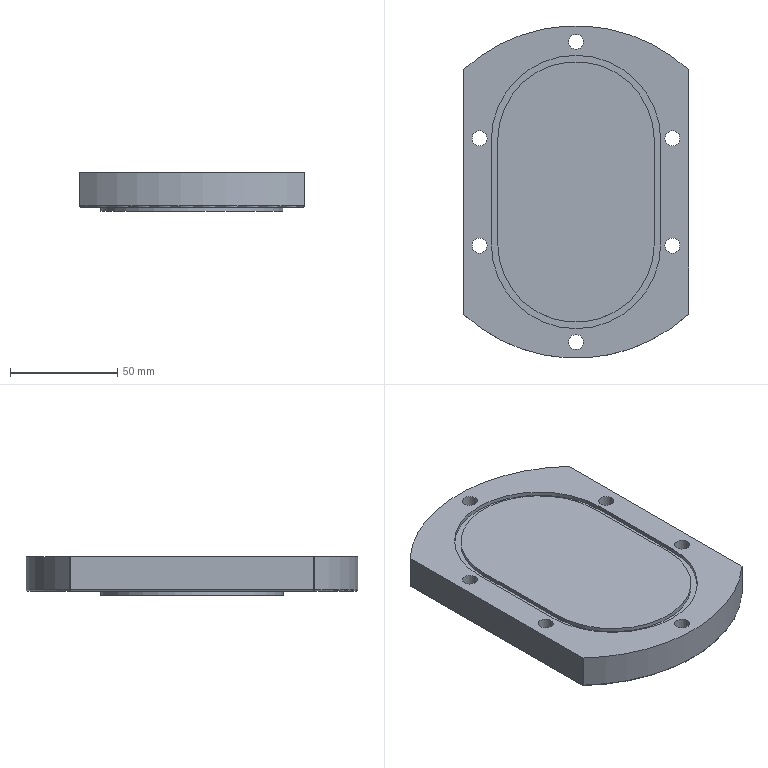NC program | NX | posted with a generic post | part box 105 x 155 x 18 mm
Whole program:
N10 G17 G21 G94 G90
(FLOOR_WALL_COPY_1_COPY , TOOL : D50)
N12 T02 M6
N14 G54
N16 G17 G0 G90 X-61.025 Y52.5 S1200 M3
N18 G43 Z30. H2
N20 Z7.65
N22 G94 G1 Z4.65 F1000.
N24 X-57.009
N26 X57.009 F2000.
N28 G2 X73.636 Y24.167 R77.5
N30 G1 X-73.636
N32 G3 X-77.388 Y-4.167 R77.5
N34 G1 X77.388
N36 G2 X70.356 Y-32.5 R77.5
N38 G1 X-70.356
N40 X-73.648
N42 Z7.65
N44 G0 Z30.
N46 X-61.025 Y52.5
N48 Z7.3
N50 G1 Z4.3 F1000.
N52 X-57.009
N54 X57.009 F2000.
N56 G2 X73.636 Y24.167 R77.5
N58 G1 X-73.636
N60 G3 X-77.388 Y-4.167 R77.5
N62 G1 X77.388
N64 G2 X70.356 Y-32.5 R77.5
N66 G1 X-70.356
N68 X-73.648
N70 Z7.3
N72 G0 Z30.
N74 X-61.025 Y52.5
N76 Z6.95
N78 G1 Z3.95 F1000.
N80 X-57.009
N82 X57.009 F2000.
N84 G2 X73.636 Y24.167 R77.5
N86 G1 X-73.636
N88 G3 X-77.388 Y-4.167 R77.5
N90 G1 X77.388
N92 G2 X70.356 Y-32.5 R77.5
N94 G1 X-70.356
N96 X-73.648
N98 Z6.95
N100 G0 Z30.
N102 X-61.025 Y52.5
N104 Z6.6
N106 G1 Z3.6 F1000.
N108 X-57.009
N110 X57.009 F2000.
N112 G2 X73.636 Y24.167 R77.5
N114 G1 X-73.636
N116 G3 X-77.388 Y-4.167 R77.5
N118 G1 X77.388
N120 G2 X70.356 Y-32.5 R77.5
N122 G1 X-70.356
N124 X-73.648
N126 Z6.6
N128 G0 Z30.
N130 X-61.025 Y52.5
N132 Z6.25
N134 G1 Z3.25 F1000.
N136 X-57.009
N138 X57.009 F2000.
N140 G2 X73.636 Y24.167 R77.5
N142 G1 X-73.636
N144 G3 X-77.388 Y-4.167 R77.5
N146 G1 X77.388
N148 G2 X70.356 Y-32.5 R77.5
N150 G1 X-70.356
N152 X-73.648
N154 Z6.25
N156 G0 Z30.
N158 X-61.025 Y52.5
N160 Z5.9
N162 G1 Z2.9 F1000.
N164 X-57.009
N166 X57.009 F2000.
N168 G2 X73.636 Y24.167 R77.5
N170 G1 X-73.636
N172 G3 X-77.388 Y-4.167 R77.5
N174 G1 X77.388
N176 G2 X70.356 Y-32.5 R77.5
N178 G1 X-70.356
N180 X-73.648
N182 Z5.9
N184 G0 Z30.
N186 X-61.025 Y52.5
N188 Z5.55
N190 G1 Z2.55 F1000.
N192 X-57.009
N194 X57.009 F2000.
N196 G2 X73.636 Y24.167 R77.5
N198 G1 X-73.636
N200 G3 X-77.388 Y-4.167 R77.5
N202 G1 X77.388
N204 G2 X70.356 Y-32.5 R77.5
N206 G1 X-70.356
N208 X-73.648
N210 Z5.55
N212 G0 Z30.
N214 X-61.025 Y52.5
N216 Z5.2
N218 G1 Z2.2 F1000.
N220 X-57.009
N222 X57.009 F2000.
N224 G2 X73.636 Y24.167 R77.5
N226 G1 X-73.636
N228 G3 X-77.388 Y-4.167 R77.5
N230 G1 X77.388
N232 G2 X70.356 Y-32.5 R77.5
N234 G1 X-70.356
N236 X-73.648
N238 Z5.2
N240 G0 Z30.
N242 X-61.025 Y52.5
N244 Z4.85
N246 G1 Z1.85 F1000.
N248 X-57.009
N250 X57.009 F2000.
N252 G2 X73.636 Y24.167 R77.5
N254 G1 X-73.636
N256 G3 X-77.388 Y-4.167 R77.5
N258 G1 X77.388
N260 G2 X70.356 Y-32.5 R77.5
N262 G1 X-70.356
N264 X-73.648
N266 Z4.85
N268 G0 Z30.
N270 X-61.025 Y52.5
N272 Z4.5
N274 G1 Z1.5 F1000.
N276 X-57.009
N278 X57.009 F2000.
N280 G2 X73.636 Y24.167 R77.5
N282 G1 X-73.636
N284 G3 X-77.388 Y-4.167 R77.5
N286 G1 X77.388
N288 G2 X70.356 Y-32.5 R77.5
N290 G1 X-70.356
N292 X-73.648
N294 Z4.5
N296 G0 Z30.
N298 X-61.025 Y52.5
N300 Z4.15
N302 G1 Z1.15 F1000.
N304 X-57.009
N306 X57.009 F2000.
N308 G2 X73.636 Y24.167 R77.5
N310 G1 X-73.636
N312 G3 X-77.388 Y-4.167 R77.5
N314 G1 X77.388
N316 G2 X70.356 Y-32.5 R77.5
N318 G1 X-70.356
N320 X-73.648
N322 Z4.15
N324 G0 Z30.
N326 X-61.025 Y52.5
N328 Z3.8
N330 G1 Z0.8 F1000.
N332 X-57.009
N334 X57.009 F2000.
N336 G2 X73.636 Y24.167 R77.5
N338 G1 X-73.636
N340 G3 X-77.388 Y-4.167 R77.5
N342 G1 X77.388
N344 G2 X70.356 Y-32.5 R77.5
N346 G1 X-70.356
N348 X-73.648
N350 Z3.8
N352 G0 Z30.
N354 X-61.025 Y52.5
N356 Z3.45
N358 G1 Z0.45 F1000.
N360 X-57.009
N362 X57.009 F2000.
N364 G2 X73.636 Y24.167 R77.5
N366 G1 X-73.636
N368 G3 X-77.388 Y-4.167 R77.5
N370 G1 X77.388
N372 G2 X70.356 Y-32.5 R77.5
N374 G1 X-70.356
N376 X-73.648
N378 Z3.45
N380 G0 Z30.
N382 X-61.025 Y52.5
N384 Z3.1
N386 G1 Z0.1 F1000.
N388 X-57.009
N390 X57.009 F2000.
N392 G2 X73.636 Y24.167 R77.5
N394 G1 X-73.636
N396 G3 X-77.388 Y-4.167 R77.5
N398 G1 X77.388
N400 G2 X70.356 Y-32.5 R77.5
N402 G1 X-70.356
N404 X-73.648
N406 Z3.1
N408 G0 Z30.
(FLOOR_WALL_COPY_COPY_COPY , TOOL : D50)
N410 X-61.025 Y52.5 S2500
N412 Z3.
N414 G1 Z0. F1000.
N416 X-57.009
N418 X57.009
N420 G2 X73.636 Y24.167 R77.5
N422 G1 X-73.636
N424 G3 X-77.388 Y-4.167 R77.5
N426 G1 X77.388
N428 G2 X70.356 Y-32.5 R77.5
N430 G1 X-70.356
N432 X-73.648
N434 Z3.
N436 G0 Z30.
N438 M5
(HOLE_MILLING_COPY_COPY , TOOL : D6)
N440 T06 M6
N442 G54
N444 G17 G0 G90 X-25. Y45. S4987 M3
N446 G43 Z30. H6
N448 Z-1.
N450 G94 G3 X-23.75 Y46.25 R1.25 F1500.
N452 X-25. Y47.5 R1.25
N454 X-25. Y47.5 Z-1.1 I0. J-2.5
N456 X-25. Y47.5 Z-1.2 I0. J-2.5
N458 X-25. Y47.5 Z-1.3 I0. J-2.5
N460 X-25. Y47.5 Z-1.4 I0. J-2.5
N462 X-25. Y47.5 Z-1.5 I0. J-2.5
N464 X-25. Y47.5 Z-1.6 I0. J-2.5
N466 X-25. Y47.5 Z-1.7 I0. J-2.5
N468 X-25. Y47.5 Z-1.8 I0. J-2.5
N470 X-25. Y47.5 Z-1.9 I0. J-2.5
N472 X-25. Y47.5 Z-2. I0. J-2.5
N474 X-25. Y47.5 Z-2.1 I0. J-2.5
N476 X-25. Y47.5 Z-2.2 I0. J-2.5
N478 X-25. Y47.5 Z-2.3 I0. J-2.5
N480 X-25. Y47.5 Z-2.4 I0. J-2.5
N482 X-25. Y47.5 Z-2.5 I0. J-2.5
N484 X-25. Y47.5 Z-2.6 I0. J-2.5
N486 X-25. Y47.5 Z-2.7 I0. J-2.5
N488 X-25. Y47.5 Z-2.8 I0. J-2.5
N490 X-25. Y47.5 Z-2.9 I0. J-2.5
N492 X-25. Y47.5 Z-3. I0. J-2.5
N494 X-25. Y47.5 Z-3.1 I0. J-2.5
N496 X-25. Y47.5 Z-3.2 I0. J-2.5
N498 X-25. Y47.5 Z-3.3 I0. J-2.5
N500 X-25. Y47.5 Z-3.4 I0. J-2.5
N502 X-25. Y47.5 Z-3.5 I0. J-2.5
N504 X-25. Y47.5 Z-3.6 I0. J-2.5
N506 X-25. Y47.5 Z-3.7 I0. J-2.5
N508 X-25. Y47.5 Z-3.8 I0. J-2.5
N510 X-25. Y47.5 Z-3.9 I0. J-2.5
N512 X-25. Y47.5 Z-4. I0. J-2.5
N514 X-25. Y47.5 Z-4.1 I0. J-2.5
N516 X-25. Y47.5 Z-4.2 I0. J-2.5
N518 X-25. Y47.5 Z-4.3 I0. J-2.5
N520 X-25. Y47.5 Z-4.4 I0. J-2.5
N522 X-25. Y47.5 Z-4.5 I0. J-2.5
N524 X-25. Y47.5 Z-4.6 I0. J-2.5
N526 X-25. Y47.5 Z-4.7 I0. J-2.5
N528 X-25. Y47.5 Z-4.8 I0. J-2.5
N530 X-25. Y47.5 Z-4.9 I0. J-2.5
N532 X-25. Y47.5 Z-5. I0. J-2.5
N534 X-25. Y47.5 Z-5.1 I0. J-2.5
N536 X-25. Y47.5 Z-5.2 I0. J-2.5
N538 X-25. Y47.5 Z-5.3 I0. J-2.5
N540 X-25. Y47.5 Z-5.4 I0. J-2.5
N542 X-25. Y47.5 Z-5.5 I0. J-2.5
N544 X-25. Y47.5 Z-5.6 I0. J-2.5
N546 X-25. Y47.5 Z-5.7 I0. J-2.5
N548 X-25. Y47.5 Z-5.8 I0. J-2.5
N550 X-25. Y47.5 Z-5.9 I0. J-2.5
N552 X-25. Y47.5 Z-6. I0. J-2.5
N554 X-25. Y47.5 Z-6.1 I0. J-2.5
N556 X-25. Y47.5 Z-6.2 I0. J-2.5
N558 X-25. Y47.5 Z-6.3 I0. J-2.5
N560 X-25. Y47.5 Z-6.4 I0. J-2.5
N562 X-25. Y47.5 Z-6.5 I0. J-2.5
N564 X-25. Y47.5 Z-6.6 I0. J-2.5
N566 X-25. Y47.5 Z-6.7 I0. J-2.5
N568 X-25. Y47.5 Z-6.8 I0. J-2.5
N570 X-25. Y47.5 Z-6.9 I0. J-2.5
N572 X-25. Y47.5 Z-7. I0. J-2.5
N574 X-25. Y47.5 Z-7.1 I0. J-2.5
N576 X-25. Y47.5 Z-7.2 I0. J-2.5
N578 X-25. Y47.5 Z-7.3 I0. J-2.5
N580 X-25. Y47.5 Z-7.4 I0. J-2.5
N582 X-25. Y47.5 Z-7.5 I0. J-2.5
N584 X-25. Y47.5 Z-7.6 I0. J-2.5
N586 X-25. Y47.5 Z-7.7 I0. J-2.5
N588 X-25. Y47.5 Z-7.8 I0. J-2.5
N590 X-25. Y47.5 Z-7.9 I0. J-2.5
N592 X-25. Y47.5 Z-8. I0. J-2.5
N594 X-25. Y47.5 Z-8.1 I0. J-2.5
N596 X-25. Y47.5 Z-8.2 I0. J-2.5
N598 X-25. Y47.5 Z-8.3 I0. J-2.5
N600 X-25. Y47.5 Z-8.4 I0. J-2.5
N602 X-25. Y47.5 Z-8.5 I0. J-2.5
N604 X-25. Y47.5 Z-8.6 I0. J-2.5
N606 X-25. Y47.5 Z-8.7 I0. J-2.5
N608 X-25. Y47.5 Z-8.8 I0. J-2.5
N610 X-27.5 Y45. R2.5
N612 X-25. Y47.5 R-2.5
N614 X-26.25 Y46.25 R1.25
N616 X-25. Y45. R1.25
N618 G0 Z30.
N620 X-70. Y0.
N622 Z-1.
N624 G3 X-68.75 Y1.25 R1.25
N626 X-70. Y2.5 R1.25
N628 X-70. Y2.5 Z-1.1 I0. J-2.5
N630 X-70. Y2.5 Z-1.2 I0. J-2.5
N632 X-70. Y2.5 Z-1.3 I0. J-2.5
N634 X-70. Y2.5 Z-1.4 I0. J-2.5
N636 X-70. Y2.5 Z-1.5 I0. J-2.5
N638 X-70. Y2.5 Z-1.6 I0. J-2.5
N640 X-70. Y2.5 Z-1.7 I0. J-2.5
N642 X-70. Y2.5 Z-1.8 I0. J-2.5
N644 X-70. Y2.5 Z-1.9 I0. J-2.5
N646 X-70. Y2.5 Z-2. I0. J-2.5
N648 X-70. Y2.5 Z-2.1 I0. J-2.5
N650 X-70. Y2.5 Z-2.2 I0. J-2.5
N652 X-70. Y2.5 Z-2.3 I0. J-2.5
N654 X-70. Y2.5 Z-2.4 I0. J-2.5
N656 X-70. Y2.5 Z-2.5 I0. J-2.5
N658 X-70. Y2.5 Z-2.6 I0. J-2.5
N660 X-70. Y2.5 Z-2.7 I0. J-2.5
N662 X-70. Y2.5 Z-2.8 I0. J-2.5
N664 X-70. Y2.5 Z-2.9 I0. J-2.5
N666 X-70. Y2.5 Z-3. I0. J-2.5
N668 X-70. Y2.5 Z-3.1 I0. J-2.5
N670 X-70. Y2.5 Z-3.2 I0. J-2.5
N672 X-70. Y2.5 Z-3.3 I0. J-2.5
N674 X-70. Y2.5 Z-3.4 I0. J-2.5
N676 X-70. Y2.5 Z-3.5 I0. J-2.5
N678 X-70. Y2.5 Z-3.6 I0. J-2.5
N680 X-70. Y2.5 Z-3.7 I0. J-2.5
N682 X-70. Y2.5 Z-3.8 I0. J-2.5
N684 X-70. Y2.5 Z-3.9 I0. J-2.5
N686 X-70. Y2.5 Z-4. I0. J-2.5
N688 X-70. Y2.5 Z-4.1 I0. J-2.5
N690 X-70. Y2.5 Z-4.2 I0. J-2.5
N692 X-70. Y2.5 Z-4.3 I0. J-2.5
N694 X-70. Y2.5 Z-4.4 I0. J-2.5
N696 X-70. Y2.5 Z-4.5 I0. J-2.5
N698 X-70. Y2.5 Z-4.6 I0. J-2.5
N700 X-70. Y2.5 Z-4.7 I0. J-2.5
N702 X-70. Y2.5 Z-4.8 I0. J-2.5
N704 X-70. Y2.5 Z-4.9 I0. J-2.5
N706 X-70. Y2.5 Z-5. I0. J-2.5
N708 X-70. Y2.5 Z-5.1 I0. J-2.5
N710 X-70. Y2.5 Z-5.2 I0. J-2.5
N712 X-70. Y2.5 Z-5.3 I0. J-2.5
N714 X-70. Y2.5 Z-5.4 I0. J-2.5
N716 X-70. Y2.5 Z-5.5 I0. J-2.5
N718 X-70. Y2.5 Z-5.6 I0. J-2.5
N720 X-70. Y2.5 Z-5.7 I0. J-2.5
N722 X-70. Y2.5 Z-5.8 I0. J-2.5
N724 X-70. Y2.5 Z-5.9 I0. J-2.5
N726 X-70. Y2.5 Z-6. I0. J-2.5
N728 X-70. Y2.5 Z-6.1 I0. J-2.5
N730 X-70. Y2.5 Z-6.2 I0. J-2.5
N732 X-70. Y2.5 Z-6.3 I0. J-2.5
N734 X-70. Y2.5 Z-6.4 I0. J-2.5
N736 X-70. Y2.5 Z-6.5 I0. J-2.5
N738 X-70. Y2.5 Z-6.6 I0. J-2.5
N740 X-70. Y2.5 Z-6.7 I0. J-2.5
N742 X-70. Y2.5 Z-6.8 I0. J-2.5
N744 X-70. Y2.5 Z-6.9 I0. J-2.5
N746 X-70. Y2.5 Z-7. I0. J-2.5
N748 X-70. Y2.5 Z-7.1 I0. J-2.5
N750 X-70. Y2.5 Z-7.2 I0. J-2.5
N752 X-70. Y2.5 Z-7.3 I0. J-2.5
N754 X-70. Y2.5 Z-7.4 I0. J-2.5
N756 X-70. Y2.5 Z-7.5 I0. J-2.5
N758 X-70. Y2.5 Z-7.6 I0. J-2.5
N760 X-70. Y2.5 Z-7.7 I0. J-2.5
N762 X-70. Y2.5 Z-7.8 I0. J-2.5
N764 X-70. Y2.5 Z-7.9 I0. J-2.5
N766 X-70. Y2.5 Z-8. I0. J-2.5
N768 X-70. Y2.5 Z-8.1 I0. J-2.5
N770 X-70. Y2.5 Z-8.2 I0. J-2.5
N772 X-70. Y2.5 Z-8.3 I0. J-2.5
N774 X-70. Y2.5 Z-8.4 I0. J-2.5
N776 X-70. Y2.5 Z-8.5 I0. J-2.5
N778 X-70. Y2.5 Z-8.6 I0. J-2.5
N780 X-70. Y2.5 Z-8.7 I0. J-2.5
N782 X-70. Y2.5 Z-8.8 I0. J-2.5
N784 X-72.5 Y0. R2.5
N786 X-70. Y2.5 R-2.5
N788 X-71.25 Y1.25 R1.25
N790 X-70. Y0. R1.25
N792 G0 Z30.
N794 X25. Y45.
N796 Z-1.
N798 G3 X26.25 Y46.25 R1.25
N800 X25. Y47.5 R1.25
N802 X25. Y47.5 Z-1.1 I0. J-2.5
N804 X25. Y47.5 Z-1.2 I0. J-2.5
N806 X25. Y47.5 Z-1.3 I0. J-2.5
N808 X25. Y47.5 Z-1.4 I0. J-2.5
N810 X25. Y47.5 Z-1.5 I0. J-2.5
N812 X25. Y47.5 Z-1.6 I0. J-2.5
N814 X25. Y47.5 Z-1.7 I0. J-2.5
N816 X25. Y47.5 Z-1.8 I0. J-2.5
N818 X25. Y47.5 Z-1.9 I0. J-2.5
N820 X25. Y47.5 Z-2. I0. J-2.5
N822 X25. Y47.5 Z-2.1 I0. J-2.5
N824 X25. Y47.5 Z-2.2 I0. J-2.5
N826 X25. Y47.5 Z-2.3 I0. J-2.5
N828 X25. Y47.5 Z-2.4 I0. J-2.5
N830 X25. Y47.5 Z-2.5 I0. J-2.5
N832 X25. Y47.5 Z-2.6 I0. J-2.5
N834 X25. Y47.5 Z-2.7 I0. J-2.5
N836 X25. Y47.5 Z-2.8 I0. J-2.5
N838 X25. Y47.5 Z-2.9 I0. J-2.5
N840 X25. Y47.5 Z-3. I0. J-2.5
N842 X25. Y47.5 Z-3.1 I0. J-2.5
N844 X25. Y47.5 Z-3.2 I0. J-2.5
N846 X25. Y47.5 Z-3.3 I0. J-2.5
N848 X25. Y47.5 Z-3.4 I0. J-2.5
N850 X25. Y47.5 Z-3.5 I0. J-2.5
N852 X25. Y47.5 Z-3.6 I0. J-2.5
N854 X25. Y47.5 Z-3.7 I0. J-2.5
N856 X25. Y47.5 Z-3.8 I0. J-2.5
N858 X25. Y47.5 Z-3.9 I0. J-2.5
N860 X25. Y47.5 Z-4. I0. J-2.5
N862 X25. Y47.5 Z-4.1 I0. J-2.5
N864 X25. Y47.5 Z-4.2 I0. J-2.5
N866 X25. Y47.5 Z-4.3 I0. J-2.5
N868 X25. Y47.5 Z-4.4 I0. J-2.5
N870 X25. Y47.5 Z-4.5 I0. J-2.5
N872 X25. Y47.5 Z-4.6 I0. J-2.5
N874 X25. Y47.5 Z-4.7 I0. J-2.5
N876 X25. Y47.5 Z-4.8 I0. J-2.5
N878 X25. Y47.5 Z-4.9 I0. J-2.5
N880 X25. Y47.5 Z-5. I0. J-2.5
N882 X25. Y47.5 Z-5.1 I0. J-2.5
N884 X25. Y47.5 Z-5.2 I0. J-2.5
N886 X25. Y47.5 Z-5.3 I0. J-2.5
N888 X25. Y47.5 Z-5.4 I0. J-2.5
N890 X25. Y47.5 Z-5.5 I0. J-2.5
N892 X25. Y47.5 Z-5.6 I0. J-2.5
N894 X25. Y47.5 Z-5.7 I0. J-2.5
N896 X25. Y47.5 Z-5.8 I0. J-2.5
N898 X25. Y47.5 Z-5.9 I0. J-2.5
N900 X25. Y47.5 Z-6. I0. J-2.5
N902 X25. Y47.5 Z-6.1 I0. J-2.5
N904 X25. Y47.5 Z-6.2 I0. J-2.5
N906 X25. Y47.5 Z-6.3 I0. J-2.5
N908 X25. Y47.5 Z-6.4 I0. J-2.5
N910 X25. Y47.5 Z-6.5 I0. J-2.5
N912 X25. Y47.5 Z-6.6 I0. J-2.5
N914 X25. Y47.5 Z-6.7 I0. J-2.5
N916 X25. Y47.5 Z-6.8 I0. J-2.5
N918 X25. Y47.5 Z-6.9 I0. J-2.5
N920 X25. Y47.5 Z-7. I0. J-2.5
N922 X25. Y47.5 Z-7.1 I0. J-2.5
N924 X25. Y47.5 Z-7.2 I0. J-2.5
N926 X25. Y47.5 Z-7.3 I0. J-2.5
N928 X25. Y47.5 Z-7.4 I0. J-2.5
N930 X25. Y47.5 Z-7.5 I0. J-2.5
N932 X25. Y47.5 Z-7.6 I0. J-2.5
N934 X25. Y47.5 Z-7.7 I0. J-2.5
N936 X25. Y47.5 Z-7.8 I0. J-2.5
N938 X25. Y47.5 Z-7.9 I0. J-2.5
N940 X25. Y47.5 Z-8. I0. J-2.5
N942 X25. Y47.5 Z-8.1 I0. J-2.5
N944 X25. Y47.5 Z-8.2 I0. J-2.5
N946 X25. Y47.5 Z-8.3 I0. J-2.5
N948 X25. Y47.5 Z-8.4 I0. J-2.5
N950 X25. Y47.5 Z-8.5 I0. J-2.5
N952 X25. Y47.5 Z-8.6 I0. J-2.5
N954 X25. Y47.5 Z-8.7 I0. J-2.5
N956 X25. Y47.5 Z-8.8 I0. J-2.5
N958 X22.5 Y45. R2.5
N960 X25. Y47.5 R-2.5
N962 X23.75 Y46.25 R1.25
N964 X25. Y45. R1.25
N966 G0 Z30.
N968 X70. Y0.
N970 Z-1.
N972 G3 X71.25 Y1.25 R1.25
N974 X70. Y2.5 R1.25
N976 X70. Y2.5 Z-1.1 I0. J-2.5
N978 X70. Y2.5 Z-1.2 I0. J-2.5
N980 X70. Y2.5 Z-1.3 I0. J-2.5
N982 X70. Y2.5 Z-1.4 I0. J-2.5
N984 X70. Y2.5 Z-1.5 I0. J-2.5
N986 X70. Y2.5 Z-1.6 I0. J-2.5
N988 X70. Y2.5 Z-1.7 I0. J-2.5
N990 X70. Y2.5 Z-1.8 I0. J-2.5
N992 X70. Y2.5 Z-1.9 I0. J-2.5
N994 X70. Y2.5 Z-2. I0. J-2.5
N996 X70. Y2.5 Z-2.1 I0. J-2.5
N998 X70. Y2.5 Z-2.2 I0. J-2.5
N1000 X70. Y2.5 Z-2.3 I0. J-2.5
N1002 X70. Y2.5 Z-2.4 I0. J-2.5
N1004 X70. Y2.5 Z-2.5 I0. J-2.5
N1006 X70. Y2.5 Z-2.6 I0. J-2.5
N1008 X70. Y2.5 Z-2.7 I0. J-2.5
N1010 X70. Y2.5 Z-2.8 I0. J-2.5
N1012 X70. Y2.5 Z-2.9 I0. J-2.5
N1014 X70. Y2.5 Z-3. I0. J-2.5
N1016 X70. Y2.5 Z-3.1 I0. J-2.5
N1018 X70. Y2.5 Z-3.2 I0. J-2.5
N1020 X70. Y2.5 Z-3.3 I0. J-2.5
N1022 X70. Y2.5 Z-3.4 I0. J-2.5
N1024 X70. Y2.5 Z-3.5 I0. J-2.5
N1026 X70. Y2.5 Z-3.6 I0. J-2.5
N1028 X70. Y2.5 Z-3.7 I0. J-2.5
N1030 X70. Y2.5 Z-3.8 I0. J-2.5
N1032 X70. Y2.5 Z-3.9 I0. J-2.5
N1034 X70. Y2.5 Z-4. I0. J-2.5
N1036 X70. Y2.5 Z-4.1 I0. J-2.5
N1038 X70. Y2.5 Z-4.2 I0. J-2.5
N1040 X70. Y2.5 Z-4.3 I0. J-2.5
N1042 X70. Y2.5 Z-4.4 I0. J-2.5
N1044 X70. Y2.5 Z-4.5 I0. J-2.5
N1046 X70. Y2.5 Z-4.6 I0. J-2.5
N1048 X70. Y2.5 Z-4.7 I0. J-2.5
N1050 X70. Y2.5 Z-4.8 I0. J-2.5
N1052 X70. Y2.5 Z-4.9 I0. J-2.5
N1054 X70. Y2.5 Z-5. I0. J-2.5
N1056 X70. Y2.5 Z-5.1 I0. J-2.5
N1058 X70. Y2.5 Z-5.2 I0. J-2.5
N1060 X70. Y2.5 Z-5.3 I0. J-2.5
N1062 X70. Y2.5 Z-5.4 I0. J-2.5
N1064 X70. Y2.5 Z-5.5 I0. J-2.5
N1066 X70. Y2.5 Z-5.6 I0. J-2.5
N1068 X70. Y2.5 Z-5.7 I0. J-2.5
N1070 X70. Y2.5 Z-5.8 I0. J-2.5
N1072 X70. Y2.5 Z-5.9 I0. J-2.5
N1074 X70. Y2.5 Z-6. I0. J-2.5
N1076 X70. Y2.5 Z-6.1 I0. J-2.5
N1078 X70. Y2.5 Z-6.2 I0. J-2.5
N1080 X70. Y2.5 Z-6.3 I0. J-2.5
N1082 X70. Y2.5 Z-6.4 I0. J-2.5
N1084 X70. Y2.5 Z-6.5 I0. J-2.5
N1086 X70. Y2.5 Z-6.6 I0. J-2.5
N1088 X70. Y2.5 Z-6.7 I0. J-2.5
N1090 X70. Y2.5 Z-6.8 I0. J-2.5
N1092 X70. Y2.5 Z-6.9 I0. J-2.5
N1094 X70. Y2.5 Z-7. I0. J-2.5
N1096 X70. Y2.5 Z-7.1 I0. J-2.5
N1098 X70. Y2.5 Z-7.2 I0. J-2.5
N1100 X70. Y2.5 Z-7.3 I0. J-2.5
N1102 X70. Y2.5 Z-7.4 I0. J-2.5
N1104 X70. Y2.5 Z-7.5 I0. J-2.5
N1106 X70. Y2.5 Z-7.6 I0. J-2.5
N1108 X70. Y2.5 Z-7.7 I0. J-2.5
N1110 X70. Y2.5 Z-7.8 I0. J-2.5
N1112 X70. Y2.5 Z-7.9 I0. J-2.5
N1114 X70. Y2.5 Z-8. I0. J-2.5
N1116 X70. Y2.5 Z-8.1 I0. J-2.5
N1118 X70. Y2.5 Z-8.2 I0. J-2.5
N1120 X70. Y2.5 Z-8.3 I0. J-2.5
N1122 X70. Y2.5 Z-8.4 I0. J-2.5
N1124 X70. Y2.5 Z-8.5 I0. J-2.5
N1126 X70. Y2.5 Z-8.6 I0. J-2.5
N1128 X70. Y2.5 Z-8.7 I0. J-2.5
N1130 X70. Y2.5 Z-8.8 I0. J-2.5
N1132 X67.5 Y0. R2.5
N1134 X70. Y2.5 R-2.5
N1136 X68.75 Y1.25 R1.25
N1138 X70. Y0. R1.25
N1140 G0 Z30.
N1142 X25. Y-45.
N1144 Z-1.
N1146 G3 X26.25 Y-43.75 R1.25
N1148 X25. Y-42.5 R1.25
N1150 X25. Y-42.5 Z-1.1 I0. J-2.5
N1152 X25. Y-42.5 Z-1.2 I0. J-2.5
N1154 X25. Y-42.5 Z-1.3 I0. J-2.5
N1156 X25. Y-42.5 Z-1.4 I0. J-2.5
N1158 X25. Y-42.5 Z-1.5 I0. J-2.5
N1160 X25. Y-42.5 Z-1.6 I0. J-2.5
N1162 X25. Y-42.5 Z-1.7 I0. J-2.5
N1164 X25. Y-42.5 Z-1.8 I0. J-2.5
N1166 X25. Y-42.5 Z-1.9 I0. J-2.5
N1168 X25. Y-42.5 Z-2. I0. J-2.5
N1170 X25. Y-42.5 Z-2.1 I0. J-2.5
N1172 X25. Y-42.5 Z-2.2 I0. J-2.5
N1174 X25. Y-42.5 Z-2.3 I0. J-2.5
N1176 X25. Y-42.5 Z-2.4 I0. J-2.5
N1178 X25. Y-42.5 Z-2.5 I0. J-2.5
N1180 X25. Y-42.5 Z-2.6 I0. J-2.5
N1182 X25. Y-42.5 Z-2.7 I0. J-2.5
N1184 X25. Y-42.5 Z-2.8 I0. J-2.5
N1186 X25. Y-42.5 Z-2.9 I0. J-2.5
N1188 X25. Y-42.5 Z-3. I0. J-2.5
N1190 X25. Y-42.5 Z-3.1 I0. J-2.5
N1192 X25. Y-42.5 Z-3.2 I0. J-2.5
N1194 X25. Y-42.5 Z-3.3 I0. J-2.5
N1196 X25. Y-42.5 Z-3.4 I0. J-2.5
N1198 X25. Y-42.5 Z-3.5 I0. J-2.5
N1200 X25. Y-42.5 Z-3.6 I0. J-2.5
N1202 X25. Y-42.5 Z-3.7 I0. J-2.5
N1204 X25. Y-42.5 Z-3.8 I0. J-2.5
N1206 X25. Y-42.5 Z-3.9 I0. J-2.5
N1208 X25. Y-42.5 Z-4. I0. J-2.5
N1210 X25. Y-42.5 Z-4.1 I0. J-2.5
N1212 X25. Y-42.5 Z-4.2 I0. J-2.5
N1214 X25. Y-42.5 Z-4.3 I0. J-2.5
N1216 X25. Y-42.5 Z-4.4 I0. J-2.5
N1218 X25. Y-42.5 Z-4.5 I0. J-2.5
N1220 X25. Y-42.5 Z-4.6 I0. J-2.5
N1222 X25. Y-42.5 Z-4.7 I0. J-2.5
N1224 X25. Y-42.5 Z-4.8 I0. J-2.5
N1226 X25. Y-42.5 Z-4.9 I0. J-2.5
N1228 X25. Y-42.5 Z-5. I0. J-2.5
N1230 X25. Y-42.5 Z-5.1 I0. J-2.5
N1232 X25. Y-42.5 Z-5.2 I0. J-2.5
N1234 X25. Y-42.5 Z-5.3 I0. J-2.5
N1236 X25. Y-42.5 Z-5.4 I0. J-2.5
N1238 X25. Y-42.5 Z-5.5 I0. J-2.5
N1240 X25. Y-42.5 Z-5.6 I0. J-2.5
N1242 X25. Y-42.5 Z-5.7 I0. J-2.5
N1244 X25. Y-42.5 Z-5.8 I0. J-2.5
N1246 X25. Y-42.5 Z-5.9 I0. J-2.5
N1248 X25. Y-42.5 Z-6. I0. J-2.5
N1250 X25. Y-42.5 Z-6.1 I0. J-2.5
N1252 X25. Y-42.5 Z-6.2 I0. J-2.5
N1254 X25. Y-42.5 Z-6.3 I0. J-2.5
N1256 X25. Y-42.5 Z-6.4 I0. J-2.5
N1258 X25. Y-42.5 Z-6.5 I0. J-2.5
N1260 X25. Y-42.5 Z-6.6 I0. J-2.5
N1262 X25. Y-42.5 Z-6.7 I0. J-2.5
N1264 X25. Y-42.5 Z-6.8 I0. J-2.5
N1266 X25. Y-42.5 Z-6.9 I0. J-2.5
N1268 X25. Y-42.5 Z-7. I0. J-2.5
N1270 X25. Y-42.5 Z-7.1 I0. J-2.5
N1272 X25. Y-42.5 Z-7.2 I0. J-2.5
N1274 X25. Y-42.5 Z-7.3 I0. J-2.5
N1276 X25. Y-42.5 Z-7.4 I0. J-2.5
N1278 X25. Y-42.5 Z-7.5 I0. J-2.5
N1280 X25. Y-42.5 Z-7.6 I0. J-2.5
N1282 X25. Y-42.5 Z-7.7 I0. J-2.5
N1284 X25. Y-42.5 Z-7.8 I0. J-2.5
N1286 X25. Y-42.5 Z-7.9 I0. J-2.5
N1288 X25. Y-42.5 Z-8. I0. J-2.5
N1290 X25. Y-42.5 Z-8.1 I0. J-2.5
N1292 X25. Y-42.5 Z-8.2 I0. J-2.5
N1294 X25. Y-42.5 Z-8.3 I0. J-2.5
N1296 X25. Y-42.5 Z-8.4 I0. J-2.5
N1298 X25. Y-42.5 Z-8.5 I0. J-2.5
N1300 X25. Y-42.5 Z-8.6 I0. J-2.5
N1302 X25. Y-42.5 Z-8.7 I0. J-2.5
N1304 X25. Y-42.5 Z-8.8 I0. J-2.5
N1306 X22.5 Y-45. R2.5
N1308 X25. Y-42.5 R-2.5
N1310 X23.75 Y-43.75 R1.25
N1312 X25. Y-45. R1.25
N1314 G0 Z30.
N1316 X-25.
N1318 Z-1.
N1320 G3 X-23.75 Y-43.75 R1.25
N1322 X-25. Y-42.5 R1.25
N1324 X-25. Y-42.5 Z-1.1 I0. J-2.5
N1326 X-25. Y-42.5 Z-1.2 I0. J-2.5
N1328 X-25. Y-42.5 Z-1.3 I0. J-2.5
N1330 X-25. Y-42.5 Z-1.4 I0. J-2.5
N1332 X-25. Y-42.5 Z-1.5 I0. J-2.5
N1334 X-25. Y-42.5 Z-1.6 I0. J-2.5
N1336 X-25. Y-42.5 Z-1.7 I0. J-2.5
N1338 X-25. Y-42.5 Z-1.8 I0. J-2.5
N1340 X-25. Y-42.5 Z-1.9 I0. J-2.5
N1342 X-25. Y-42.5 Z-2. I0. J-2.5
N1344 X-25. Y-42.5 Z-2.1 I0. J-2.5
N1346 X-25. Y-42.5 Z-2.2 I0. J-2.5
N1348 X-25. Y-42.5 Z-2.3 I0. J-2.5
N1350 X-25. Y-42.5 Z-2.4 I0. J-2.5
N1352 X-25. Y-42.5 Z-2.5 I0. J-2.5
N1354 X-25. Y-42.5 Z-2.6 I0. J-2.5
N1356 X-25. Y-42.5 Z-2.7 I0. J-2.5
N1358 X-25. Y-42.5 Z-2.8 I0. J-2.5
N1360 X-25. Y-42.5 Z-2.9 I0. J-2.5
N1362 X-25. Y-42.5 Z-3. I0. J-2.5
N1364 X-25. Y-42.5 Z-3.1 I0. J-2.5
N1366 X-25. Y-42.5 Z-3.2 I0. J-2.5
N1368 X-25. Y-42.5 Z-3.3 I0. J-2.5
N1370 X-25. Y-42.5 Z-3.4 I0. J-2.5
N1372 X-25. Y-42.5 Z-3.5 I0. J-2.5
N1374 X-25. Y-42.5 Z-3.6 I0. J-2.5
N1376 X-25. Y-42.5 Z-3.7 I0. J-2.5
N1378 X-25. Y-42.5 Z-3.8 I0. J-2.5
N1380 X-25. Y-42.5 Z-3.9 I0. J-2.5
N1382 X-25. Y-42.5 Z-4. I0. J-2.5
N1384 X-25. Y-42.5 Z-4.1 I0. J-2.5
N1386 X-25. Y-42.5 Z-4.2 I0. J-2.5
N1388 X-25. Y-42.5 Z-4.3 I0. J-2.5
N1390 X-25. Y-42.5 Z-4.4 I0. J-2.5
N1392 X-25. Y-42.5 Z-4.5 I0. J-2.5
N1394 X-25. Y-42.5 Z-4.6 I0. J-2.5
N1396 X-25. Y-42.5 Z-4.7 I0. J-2.5
N1398 X-25. Y-42.5 Z-4.8 I0. J-2.5
N1400 X-25. Y-42.5 Z-4.9 I0. J-2.5
N1402 X-25. Y-42.5 Z-5. I0. J-2.5
N1404 X-25. Y-42.5 Z-5.1 I0. J-2.5
N1406 X-25. Y-42.5 Z-5.2 I0. J-2.5
N1408 X-25. Y-42.5 Z-5.3 I0. J-2.5
N1410 X-25. Y-42.5 Z-5.4 I0. J-2.5
N1412 X-25. Y-42.5 Z-5.5 I0. J-2.5
N1414 X-25. Y-42.5 Z-5.6 I0. J-2.5
N1416 X-25. Y-42.5 Z-5.7 I0. J-2.5
N1418 X-25. Y-42.5 Z-5.8 I0. J-2.5
N1420 X-25. Y-42.5 Z-5.9 I0. J-2.5
N1422 X-25. Y-42.5 Z-6. I0. J-2.5
N1424 X-25. Y-42.5 Z-6.1 I0. J-2.5
N1426 X-25. Y-42.5 Z-6.2 I0. J-2.5
N1428 X-25. Y-42.5 Z-6.3 I0. J-2.5
N1430 X-25. Y-42.5 Z-6.4 I0. J-2.5
N1432 X-25. Y-42.5 Z-6.5 I0. J-2.5
N1434 X-25. Y-42.5 Z-6.6 I0. J-2.5
N1436 X-25. Y-42.5 Z-6.7 I0. J-2.5
N1438 X-25. Y-42.5 Z-6.8 I0. J-2.5
N1440 X-25. Y-42.5 Z-6.9 I0. J-2.5
N1442 X-25. Y-42.5 Z-7. I0. J-2.5
N1444 X-25. Y-42.5 Z-7.1 I0. J-2.5
N1446 X-25. Y-42.5 Z-7.2 I0. J-2.5
N1448 X-25. Y-42.5 Z-7.3 I0. J-2.5
N1450 X-25. Y-42.5 Z-7.4 I0. J-2.5
N1452 X-25. Y-42.5 Z-7.5 I0. J-2.5
N1454 X-25. Y-42.5 Z-7.6 I0. J-2.5
N1456 X-25. Y-42.5 Z-7.7 I0. J-2.5
N1458 X-25. Y-42.5 Z-7.8 I0. J-2.5
N1460 X-25. Y-42.5 Z-7.9 I0. J-2.5
N1462 X-25. Y-42.5 Z-8. I0. J-2.5
N1464 X-25. Y-42.5 Z-8.1 I0. J-2.5
N1466 X-25. Y-42.5 Z-8.2 I0. J-2.5
N1468 X-25. Y-42.5 Z-8.3 I0. J-2.5
N1470 X-25. Y-42.5 Z-8.4 I0. J-2.5
N1472 X-25. Y-42.5 Z-8.5 I0. J-2.5
N1474 X-25. Y-42.5 Z-8.6 I0. J-2.5
N1476 X-25. Y-42.5 Z-8.7 I0. J-2.5
N1478 X-25. Y-42.5 Z-8.8 I0. J-2.5
N1480 X-27.5 Y-45. R2.5
N1482 X-25. Y-42.5 R-2.5
N1484 X-26.25 Y-43.75 R1.25
N1486 X-25. Y-45. R1.25
N1488 G0 Z30.
N1490 M5
(PLANAR_MILL_COPY_COPY_COPY , TOOL : D6A45)
N1492 T07 M6
N1494 G54
N1496 G17 G0 G90 X-0.766 Y44.157 S7500 M3
N1498 G43 Z30. H7
N1500 Z1.5
N1502 G94 G1 Z-1.5 F1250.
N1504 G3 X0. Y43.8 R1.
N1506 G2 X43.8 Y0. R43.8
N1508 X0. Y43.8 R-43.8
N1510 G3 X0.766 Y44.157 R1.
N1512 G1 Z1.5
N1514 G0 Z30.
(PLANAR_MILL_COPY_COPY_COPY_COPY , TOOL : D6A45)
N1516 X73.843 Y-0.766
N1518 Z-0.5
N1520 G1 Z-3.5
N1522 G3 X74.2 Y0. R1.
N1524 X70. Y4.2 R4.2
N1526 X74.2 Y0. R-4.2
N1528 X73.843 Y0.766 R1.
N1530 G1 Z-0.5
N1532 G0 Z30.
N1534 X24.234 Y-48.843
N1536 Z-0.5
N1538 G1 Z-3.5
N1540 G3 X25. Y-49.2 R1.
N1542 X29.2 Y-45. R4.2
N1544 X25. Y-49.2 R-4.2
N1546 X25.766 Y-48.843 R1.
N1548 G1 Z-0.5
N1550 G0 Z30.
N1552 X-25.766
N1554 Z-0.5
N1556 G1 Z-3.5
N1558 G3 X-25. Y-49.2 R1.
N1560 X-20.8 Y-45. R4.2
N1562 X-25. Y-49.2 R-4.2
N1564 X-24.234 Y-48.843 R1.
N1566 G1 Z-0.5
N1568 G0 Z30.
N1570 X0.766 Y-54.157
N1572 Z-0.5
N1574 G1 Z-3.5
N1576 G3 X0. Y-53.8 R1.
N1578 G1 X-56.789
N1580 G2 X-58.117 Y-53.216 R1.8
N1582 X-57.965 Y53.381 R78.8
N1584 X-57.009 Y53.8 R1.3
N1586 G1 X56.789
N1588 G2 X58.117 Y53.216 R1.8
N1590 X58.117 Y-53.216 R78.8
N1592 X56.789 Y-53.8 R1.8
N1594 G1 X0.
N1596 G3 X-0.766 Y-54.157 R1.
N1598 G1 Z-0.5
N1600 G0 Z30.
N1602 X25.766 Y48.843
N1604 Z-0.5
N1606 G1 Z-3.5
N1608 G3 X25. Y49.2 R1.
N1610 X20.8 Y45. R4.2
N1612 X25. Y49.2 R-4.2
N1614 X24.234 Y48.843 R1.
N1616 G1 Z-0.5
N1618 G0 Z30.
N1620 X-24.234
N1622 Z-0.5
N1624 G1 Z-3.5
N1626 G3 X-25. Y49.2 R1.
N1628 X-29.2 Y45. R4.2
N1630 X-25. Y49.2 R-4.2
N1632 X-25.766 Y48.843 R1.
N1634 G1 Z-0.5
N1636 G0 Z30.
N1638 X-73.843 Y0.766
N1640 Z-0.5
N1642 G1 Z-3.5
N1644 G3 X-74.2 Y0. R1.
N1646 X-70. Y-4.2 R4.2
N1648 X-74.2 Y0. R-4.2
N1650 X-73.843 Y-0.766 R1.
N1652 G1 Z-0.5
N1654 G0 Z30.
N1656 M5
N1658 M2